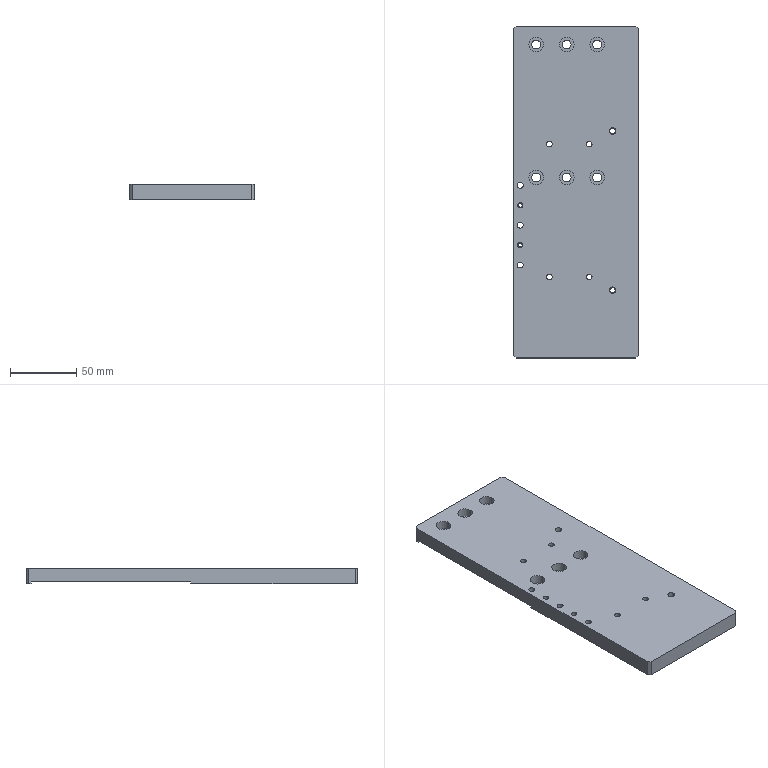Part | STEP file | 1 solid | 115 faces | box 94 x 250 x 12 mm | volume 257525 mm3 | cylinder 74 | plane 27 | cone 14 | commonest cylinder face diameters 3.3 x14 6.6 x12 11 x12 4 x8 4.2 x8 4.5 x6